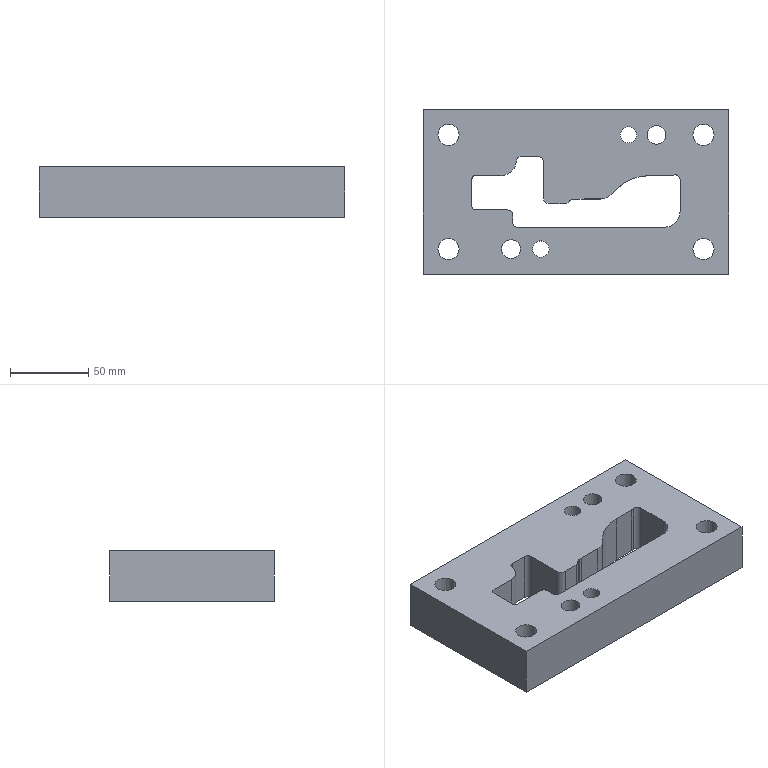Part | STEP file | lll_id258_x_t | 1 solid | 55 faces | box 195 x 105 x 32 mm | volume 501222 mm3 | cylinder 32 | plane 23 | commonest cylinder face diameters 6 x6 13.509 x4 20.008 x4 20 x3 4 x2 8 x2